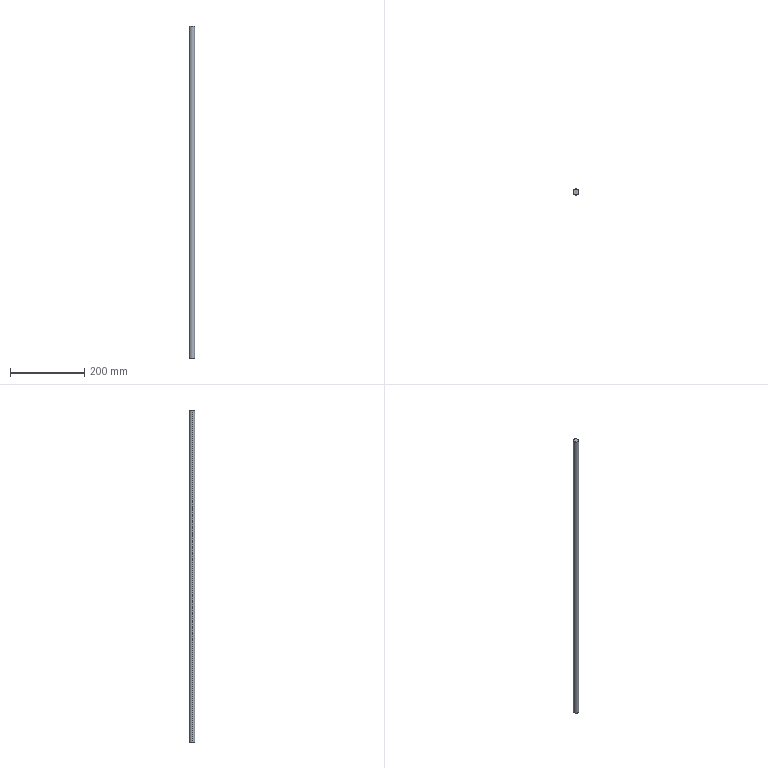Part | SolidWorks | features BaseBody 1 | 1 solid | 4 faces | box 15 x 15 x 892 mm | volume 157629 mm3 | cylinder 2 | plane 2 | commonest cylinder face diameters 15 x2
STEP:
#1=CARTESIAN_POINT('',(150.547,1879.544,-332.));
#2=VERTEX_POINT('',#1);
#3=CARTESIAN_POINT('',(165.547,1879.544,-332.));
#4=VERTEX_POINT('',#3);
#5=CARTESIAN_POINT('',(158.047,1879.544,-332.));
#6=DIRECTION('',(0.,0.,-1.));
#7=DIRECTION('',(-1.,0.,0.));
#8=AXIS2_PLACEMENT_3D('',#5,#6,#7);
#9=CIRCLE('',#8,7.5);
#10=EDGE_CURVE('',#2,#4,#9,.T.);
#11=ORIENTED_EDGE('',*,*,#10,.T.);
#12=CARTESIAN_POINT('',(165.547,1879.544,-1224.));
#13=VERTEX_POINT('',#12);
#14=CARTESIAN_POINT('',(165.547,1879.544,-424.));
#15=DIRECTION('',(0.,0.,-1.));
#16=VECTOR('',#15,1000.);
#17=LINE('',#14,#16);
#18=EDGE_CURVE('',#4,#13,#17,.T.);
#19=ORIENTED_EDGE('',*,*,#18,.T.);
#20=CARTESIAN_POINT('',(150.547,1879.544,-1224.));
#21=VERTEX_POINT('',#20);
#22=CARTESIAN_POINT('',(158.047,1879.544,-1224.));
#23=DIRECTION('',(0.,0.,1.));
#24=DIRECTION('',(-1.,0.,0.));
#25=AXIS2_PLACEMENT_3D('',#22,#23,#24);
#26=CIRCLE('',#25,7.5);
#27=EDGE_CURVE('',#13,#21,#26,.T.);
#28=ORIENTED_EDGE('',*,*,#27,.T.);
#29=CARTESIAN_POINT('',(150.547,1879.544,-424.));
#30=DIRECTION('',(0.,0.,-1.));
#31=VECTOR('',#30,1000.);
#32=LINE('',#29,#31);
#33=EDGE_CURVE('',#2,#21,#32,.T.);
#34=ORIENTED_EDGE('',*,*,#33,.F.);
#35=EDGE_LOOP('',(#11,#19,#28,#34));
#36=FACE_OUTER_BOUND('',#35,.T.);
#37=CARTESIAN_POINT('',(158.047,1879.544,-424.));
#38=DIRECTION('',(0.,0.,-1.));
#39=DIRECTION('',(-1.,0.,0.));
#40=AXIS2_PLACEMENT_3D('',#37,#38,#39);
#41=CYLINDRICAL_SURFACE('',#40,7.5);
#42=ADVANCED_FACE('',(#36),#41,.T.);
#43=ORIENTED_EDGE('',*,*,#18,.F.);
#44=CARTESIAN_POINT('',(158.047,1879.544,-332.));
#45=DIRECTION('',(0.,0.,-1.));
#46=DIRECTION('',(-1.,0.,0.));
#47=AXIS2_PLACEMENT_3D('',#44,#45,#46);
#48=CIRCLE('',#47,7.5);
#49=EDGE_CURVE('',#4,#2,#48,.T.);
#50=ORIENTED_EDGE('',*,*,#49,.T.);
#51=ORIENTED_EDGE('',*,*,#33,.T.);
#52=CARTESIAN_POINT('',(158.047,1879.544,-1224.));
#53=DIRECTION('',(0.,0.,1.));
#54=DIRECTION('',(-1.,0.,0.));
#55=AXIS2_PLACEMENT_3D('',#52,#53,#54);
#56=CIRCLE('',#55,7.5);
#57=EDGE_CURVE('',#21,#13,#56,.T.);
#58=ORIENTED_EDGE('',*,*,#57,.T.);
#59=EDGE_LOOP('',(#43,#50,#51,#58));
#60=FACE_OUTER_BOUND('',#59,.T.);
#61=CARTESIAN_POINT('',(158.047,1879.544,-424.));
#62=DIRECTION('',(0.,0.,-1.));
#63=DIRECTION('',(-1.,0.,0.));
#64=AXIS2_PLACEMENT_3D('',#61,#62,#63);
#65=CYLINDRICAL_SURFACE('',#64,7.5);
#66=ADVANCED_FACE('',(#60),#65,.T.);
#67=ORIENTED_EDGE('',*,*,#10,.F.);
#68=ORIENTED_EDGE('',*,*,#49,.F.);
#69=EDGE_LOOP('',(#67,#68));
#70=FACE_OUTER_BOUND('',#69,.T.);
#71=CARTESIAN_POINT('',(158.047,1879.544,-332.));
#72=DIRECTION('',(0.,0.,1.));
#73=DIRECTION('',(1.,0.,0.));
#74=AXIS2_PLACEMENT_3D('',#71,#72,#73);
#75=PLANE('',#74);
#76=ADVANCED_FACE('',(#70),#75,.T.);
#77=ORIENTED_EDGE('',*,*,#57,.F.);
#78=ORIENTED_EDGE('',*,*,#27,.F.);
#79=EDGE_LOOP('',(#77,#78));
#80=FACE_OUTER_BOUND('',#79,.T.);
#81=CARTESIAN_POINT('',(158.047,1879.544,-1224.));
#82=DIRECTION('',(0.,0.,1.));
#83=DIRECTION('',(1.,0.,0.));
#84=AXIS2_PLACEMENT_3D('',#81,#82,#83);
#85=PLANE('',#84);
#86=ADVANCED_FACE('',(#80),#85,.F.);
#87=CLOSED_SHELL('',(#42,#66,#76,#86));
#88=MANIFOLD_SOLID_BREP('',#87);
#89=CARTESIAN_POINT('',(0.,0.,0.));
#90=DIRECTION('',(0.,0.,1.));
#91=DIRECTION('',(1.,0.,0.));
#92=AXIS2_PLACEMENT_3D('',#89,#90,#91);
#93=(LENGTH_UNIT()NAMED_UNIT(*)SI_UNIT(.MILLI.,.METRE.));
#94=UNCERTAINTY_MEASURE_WITH_UNIT(LENGTH_MEASURE(0.00001),#93,'','');
#95=(NAMED_UNIT(*)PLANE_ANGLE_UNIT()SI_UNIT($,.RADIAN.));
#96=(NAMED_UNIT(*)SI_UNIT($,.STERADIAN.)SOLID_ANGLE_UNIT());
#97=(GEOMETRIC_REPRESENTATION_CONTEXT(3)GLOBAL_UNCERTAINTY_ASSIGNED_CONTEXT((#94))GLOBAL_UNIT_ASSIGNED_CONTEXT((#93,#95,#96))REPRESENTATION_CONTEXT('',''));
#98=ADVANCED_BREP_SHAPE_REPRESENTATION('',(#88,#92),#97);